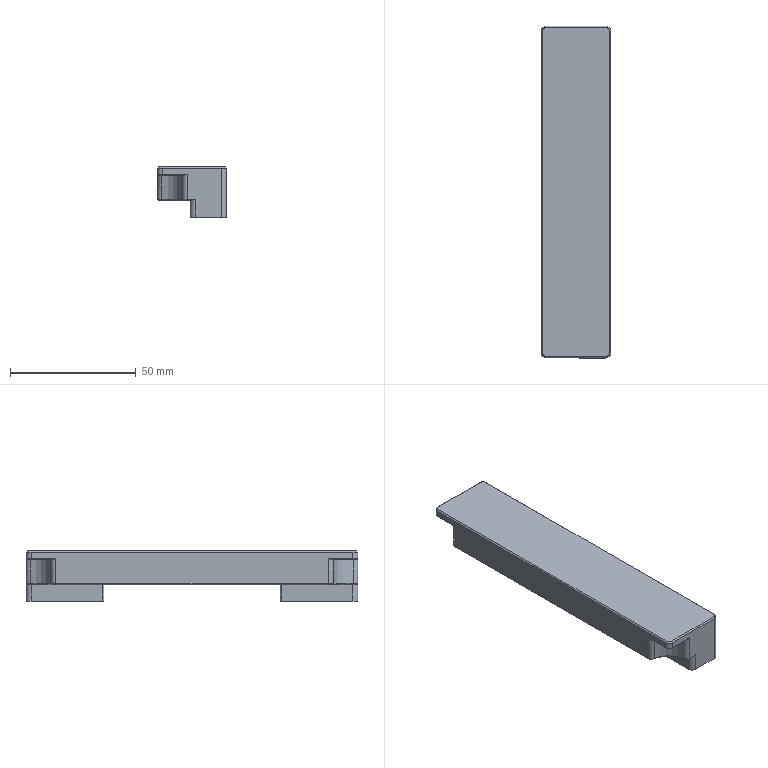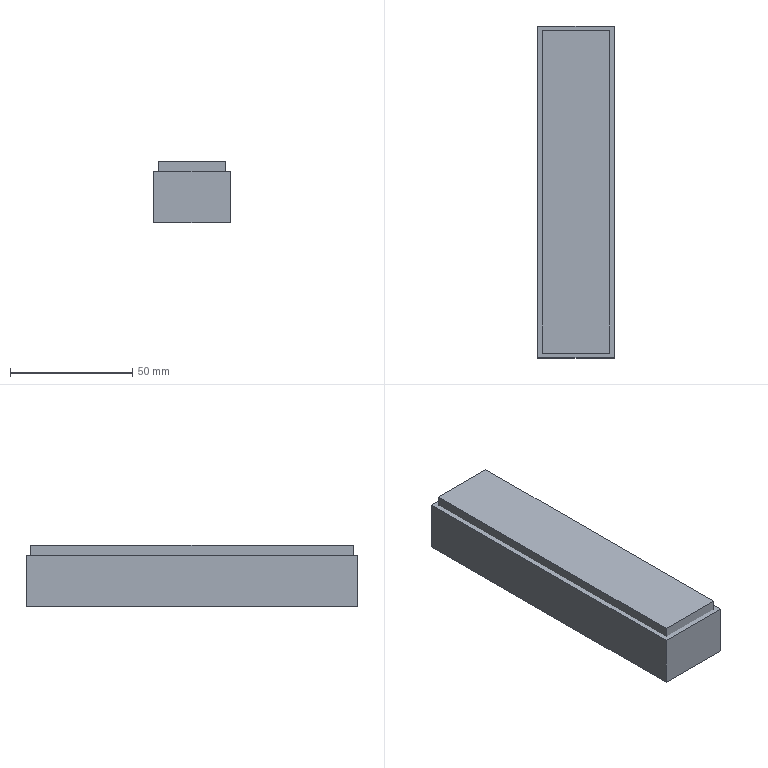CAM job | NX | 3-axis milling | part box 27.5 x 132 x 20 mm | stock box 31.5 x 136 x 25 mm
Tools:
number,name,description,diameter,corner_radius,flute_length,length,flutes
19,D80,Milling Tool-5 Parameters,80.0,0.0,50.0,75.0,2
15,D10,Milling Tool-5 Parameters,10.0,0.0,50.0,75.0,2
14,D10JING,Milling Tool-5 Parameters,10.0,0.0,50.0,75.0,2
11,D4,Milling Tool-5 Parameters,4.0,0.0,50.0,75.0,2
1,D6A45,Milling Tool-5 Parameters,6.0,0.0,50.0,75.0,2
Operations:
program,operation,operation_type,tool,method,geometry_group,spindle_rpm,surface_speed,feed_per_tooth,feed_cut,feed_plunge,cut_length_mm,path_length_mm,cut_time_min,machine_time_min
1,FLOOR_WALL,VolumeBased25DMillingOperation,D80,METHOD,A,6500.0,1633.0,0.1154,1500.0,100.0,228.0,282.0,0.152,0.1574
1,ZLEVEL_PROFILE_COPY_1,ZLevelMilling,D10,METHOD,A,9500.0,298.0,0.1842,3500.0,1000.0,7348.85,7425.85,2.134,2.142
1,FLOOR_WALL_1,VolumeBased25DMillingOperation,D10,METHOD,A,9500.0,298.0,0.1316,2500.0,100.0,1863.392,1950.192,0.7454,0.754
1,FLOOR_WALL_1_COPY,VolumeBased25DMillingOperation,D10,METHOD,A,9500.0,298.0,0.1316,2500.0,100.0,492.123,807.865,0.1968,0.2284
1,FLOOR_WALL_1_COPY_1,VolumeBased25DMillingOperation,D10,METHOD,A,9500.0,298.0,0.1316,2500.0,100.0,4264.426,4657.219,1.706,1.745
1,ZLEVEL_PROFILE_COPY_1_COPY,ZLevelMilling,D10JING,METHOD,A,9500.0,298.0,0.0632,1200.0,1000.0,1263.436,1340.936,1.089,1.097
1,FLOOR_WALL_2,VolumeBased25DMillingOperation,D10JING,METHOD,A,9500.0,298.0,0.0789,1500.0,100.0,1061.053,2696.932,0.7074,0.871
1,HOLE_MILLING,CylinderMilling,D4,METHOD,A,9500.0,119.0,0.0658,1250.0,100.0,777.468,1218.477,0.622,0.6661
1,ZLEVEL_PROFILE_COPY_1_COPY_1,ZLevelMilling,D4,METHOD,A,9500.0,298.0,0.0947,1800.0,1000.0,354.683,782.537,0.2115,0.2543
1,PLANAR_MILL_COPY_COPY_COPY_COPY_COPY_COPY_COPY_COPY_1,PlanarMilling,D6A45,METHOD,A,9500.0,179.0,0.0658,1250.0,100.0,207.261,424.262,0.1658,0.1875
1,PLANAR_MILL_COPY_COPY_COPY_COPY,PlanarMilling,D6A45,METHOD,A,9500.0,179.0,0.0658,1250.0,100.0,45.123,284.089,0.0361,0.06
1,PLANAR_MILL_COPY_COPY_COPY_COPY_COPY,PlanarMilling,D6A45,METHOD,A,9500.0,179.0,0.0658,1250.0,100.0,196.054,468.519,0.1568,0.1841
1,PLANAR_MILL_COPY_COPY_COPY_COPY_COPY_COPY,PlanarMilling,D6A45,METHOD,A,9500.0,179.0,0.0658,1250.0,100.0,43.23,347.296,0.0346,0.065
1,PLANAR_MILL_COPY_COPY_COPY_COPY_COPY_COPY_COPY,PlanarMilling,D6A45,METHOD,A,9500.0,179.0,0.0658,1250.0,100.0,70.296,143.296,0.0562,0.0635
1,PLANAR_MILL_COPY_COPY_COPY_COPY_COPY_COPY_COPY_COPY,PlanarMilling,D6A45,METHOD,A,9500.0,179.0,0.0658,1250.0,100.0,71.811,164.811,0.0574,0.0667
1,HOLE_MILLING_COPY,CylinderMilling,D4,METHOD,A,9500.0,119.0,0.0658,1250.0,100.0,192.743,633.752,0.1542,0.1983
2,FLOOR_WALL_COPY,VolumeBased25DMillingOperation,D80,METHOD,B,6500.0,1633.0,0.1154,1500.0,100.0,1120.0,2242.001,0.7467,0.8589
2,PLANAR_MILL_COPY_COPY_COPY_COPY_COPY_1,PlanarMilling,D6A45,METHOD,B,9500.0,179.0,0.0658,1250.0,100.0,328.56,388.56,0.2628,0.2688